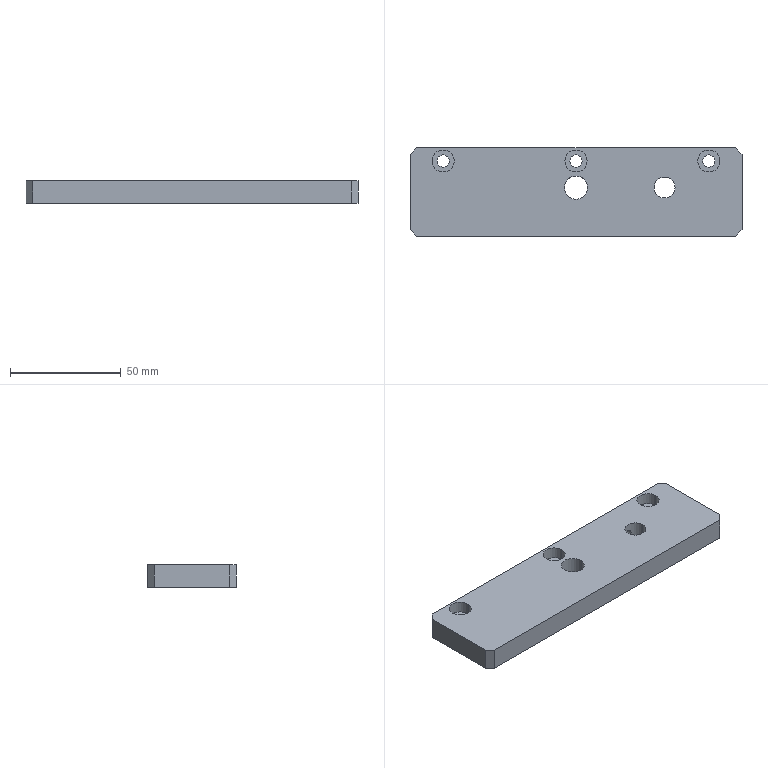Part | SolidWorks | features HoleWzd 3, Chamfer 1, Extrusion 1, ICE 1 | 1 solid | 31 faces | box 150 x 40 x 10 mm | volume 56531 mm3 | cylinder 18 | plane 13 | commonest cylinder face diameters 5.5 x6 10 x6 3.3 x2 9.5 x2 10.5 x2
STEP:
#1=CARTESIAN_POINT('',(40.,6.75,3.35));
#2=VERTEX_POINT('',#1);
#3=CARTESIAN_POINT('',(40.,6.75,6.65));
#4=VERTEX_POINT('',#3);
#5=CARTESIAN_POINT('',(40.,6.75,3.35));
#6=CARTESIAN_POINT('',(39.783,6.75,3.35));
#7=CARTESIAN_POINT('',(39.565,6.734,3.394));
#8=CARTESIAN_POINT('',(39.266,6.694,3.518));
#9=CARTESIAN_POINT('',(39.17,6.678,3.57));
#10=CARTESIAN_POINT('',(38.992,6.643,3.69));
#11=CARTESIAN_POINT('',(38.909,6.624,3.757));
#12=CARTESIAN_POINT('',(38.68,6.566,3.986));
#13=CARTESIAN_POINT('',(38.56,6.527,4.166));
#14=CARTESIAN_POINT('',(38.435,6.485,4.466));
#15=CARTESIAN_POINT('',(38.403,6.474,4.569));
#16=CARTESIAN_POINT('',(38.361,6.458,4.781));
#17=CARTESIAN_POINT('',(38.35,6.454,4.892));
#18=CARTESIAN_POINT('',(38.35,6.454,5.109));
#19=CARTESIAN_POINT('',(38.361,6.458,5.217));
#20=CARTESIAN_POINT('',(38.403,6.474,5.43));
#21=CARTESIAN_POINT('',(38.436,6.485,5.535));
#22=CARTESIAN_POINT('',(38.56,6.527,5.833));
#23=CARTESIAN_POINT('',(38.682,6.566,6.015));
#24=CARTESIAN_POINT('',(38.909,6.624,6.242));
#25=CARTESIAN_POINT('',(38.993,6.643,6.312));
#26=CARTESIAN_POINT('',(39.171,6.678,6.431));
#27=CARTESIAN_POINT('',(39.266,6.694,6.481));
#28=CARTESIAN_POINT('',(39.465,6.721,6.565));
#29=CARTESIAN_POINT('',(39.57,6.732,6.597));
#30=CARTESIAN_POINT('',(39.782,6.746,6.639));
#31=CARTESIAN_POINT('',(39.89,6.75,6.65));
#32=CARTESIAN_POINT('',(40.,6.75,6.65));
#33=B_SPLINE_CURVE_WITH_KNOTS('',3,(#5,#6,#7,#8,#9,#10,#11,#12,#13,#14,#15,#16,#17,#18,#19,#20,#21,#22,#23,#24,#25,#26,#27,#28,#29,#30,#31,#32),.UNSPECIFIED.,.F.,.F.,(4,2,2,2,2,2,2,2,2,2,2,2,2,4),(0.0052,0.005849,0.006174,0.006499,0.007149,0.007474,0.007799,0.008124,0.008448,0.009098,0.009423,0.009748,0.01007,0.0104),.UNSPECIFIED.);
#34=EDGE_CURVE('',#2,#4,#33,.T.);
#35=ORIENTED_EDGE('',*,*,#34,.F.);
#36=CARTESIAN_POINT('',(40.,20.,3.35));
#37=VERTEX_POINT('',#36);
#38=CARTESIAN_POINT('',(40.,20.,3.35));
#39=DIRECTION('',(0.,1.,0.));
#40=VECTOR('',#39,1000.);
#41=LINE('',#38,#40);
#42=EDGE_CURVE('',#2,#37,#41,.T.);
#43=ORIENTED_EDGE('',*,*,#42,.T.);
#44=CARTESIAN_POINT('',(40.,20.,6.65));
#45=VERTEX_POINT('',#44);
#46=CARTESIAN_POINT('',(40.,20.,5.));
#47=DIRECTION('',(0.,1.,0.));
#48=DIRECTION('',(0.,0.,1.));
#49=AXIS2_PLACEMENT_3D('',#46,#47,#48);
#50=CIRCLE('',#49,1.65);
#51=EDGE_CURVE('',#37,#45,#50,.T.);
#52=ORIENTED_EDGE('',*,*,#51,.T.);
#53=CARTESIAN_POINT('',(40.,20.,6.65));
#54=DIRECTION('',(0.,1.,0.));
#55=VECTOR('',#54,1000.);
#56=LINE('',#53,#55);
#57=EDGE_CURVE('',#4,#45,#56,.T.);
#58=ORIENTED_EDGE('',*,*,#57,.F.);
#59=EDGE_LOOP('',(#35,#43,#52,#58));
#60=FACE_OUTER_BOUND('',#59,.T.);
#61=CARTESIAN_POINT('',(40.,20.,5.));
#62=DIRECTION('',(0.,1.,0.));
#63=DIRECTION('',(0.,0.,1.));
#64=AXIS2_PLACEMENT_3D('',#61,#62,#63);
#65=CYLINDRICAL_SURFACE('',#64,1.65);
#66=ADVANCED_FACE('',(#60),#65,.F.);
#67=CARTESIAN_POINT('',(55.,14.,4.6));
#68=VERTEX_POINT('',#67);
#69=CARTESIAN_POINT('',(65.,14.,4.6));
#70=VERTEX_POINT('',#69);
#71=CARTESIAN_POINT('',(60.,14.,4.6));
#72=DIRECTION('',(0.,0.,1.));
#73=DIRECTION('',(1.,0.,0.));
#74=AXIS2_PLACEMENT_3D('',#71,#72,#73);
#75=CIRCLE('',#74,5.);
#76=EDGE_CURVE('',#68,#70,#75,.T.);
#77=ORIENTED_EDGE('',*,*,#76,.F.);
#78=CARTESIAN_POINT('',(55.,14.,10.));
#79=VERTEX_POINT('',#78);
#80=CARTESIAN_POINT('',(55.,14.,10.));
#81=DIRECTION('',(0.,0.,1.));
#82=VECTOR('',#81,1000.);
#83=LINE('',#80,#82);
#84=EDGE_CURVE('',#68,#79,#83,.T.);
#85=ORIENTED_EDGE('',*,*,#84,.T.);
#86=CARTESIAN_POINT('',(65.,14.,10.));
#87=VERTEX_POINT('',#86);
#88=CARTESIAN_POINT('',(60.,14.,10.));
#89=DIRECTION('',(0.,0.,1.));
#90=DIRECTION('',(1.,0.,0.));
#91=AXIS2_PLACEMENT_3D('',#88,#89,#90);
#92=CIRCLE('',#91,5.);
#93=EDGE_CURVE('',#79,#87,#92,.T.);
#94=ORIENTED_EDGE('',*,*,#93,.T.);
#95=CARTESIAN_POINT('',(65.,14.,10.));
#96=DIRECTION('',(0.,0.,1.));
#97=VECTOR('',#96,1000.);
#98=LINE('',#95,#97);
#99=EDGE_CURVE('',#70,#87,#98,.T.);
#100=ORIENTED_EDGE('',*,*,#99,.F.);
#101=EDGE_LOOP('',(#77,#85,#94,#100));
#102=FACE_OUTER_BOUND('',#101,.T.);
#103=CARTESIAN_POINT('',(60.,14.,10.));
#104=DIRECTION('',(0.,0.,1.));
#105=DIRECTION('',(1.,0.,0.));
#106=AXIS2_PLACEMENT_3D('',#103,#104,#105);
#107=CYLINDRICAL_SURFACE('',#106,5.);
#108=ADVANCED_FACE('',(#102),#107,.F.);
#109=CARTESIAN_POINT('',(57.25,14.,0.));
#110=VERTEX_POINT('',#109);
#111=CARTESIAN_POINT('',(62.75,14.,0.));
#112=VERTEX_POINT('',#111);
#113=CARTESIAN_POINT('',(60.,14.,0.));
#114=DIRECTION('',(0.,0.,1.));
#115=DIRECTION('',(1.,0.,0.));
#116=AXIS2_PLACEMENT_3D('',#113,#114,#115);
#117=CIRCLE('',#116,2.75);
#118=EDGE_CURVE('',#110,#112,#117,.T.);
#119=ORIENTED_EDGE('',*,*,#118,.F.);
#120=CARTESIAN_POINT('',(57.25,14.,4.6));
#121=VERTEX_POINT('',#120);
#122=CARTESIAN_POINT('',(57.25,14.,10.));
#123=DIRECTION('',(0.,0.,1.));
#124=VECTOR('',#123,1000.);
#125=LINE('',#122,#124);
#126=EDGE_CURVE('',#110,#121,#125,.T.);
#127=ORIENTED_EDGE('',*,*,#126,.T.);
#128=CARTESIAN_POINT('',(62.75,14.,4.6));
#129=VERTEX_POINT('',#128);
#130=CARTESIAN_POINT('',(60.,14.,4.6));
#131=DIRECTION('',(0.,0.,1.));
#132=DIRECTION('',(1.,0.,0.));
#133=AXIS2_PLACEMENT_3D('',#130,#131,#132);
#134=CIRCLE('',#133,2.75);
#135=EDGE_CURVE('',#121,#129,#134,.T.);
#136=ORIENTED_EDGE('',*,*,#135,.T.);
#137=CARTESIAN_POINT('',(62.75,14.,10.));
#138=DIRECTION('',(0.,0.,1.));
#139=VECTOR('',#138,1000.);
#140=LINE('',#137,#139);
#141=EDGE_CURVE('',#112,#129,#140,.T.);
#142=ORIENTED_EDGE('',*,*,#141,.F.);
#143=EDGE_LOOP('',(#119,#127,#136,#142));
#144=FACE_OUTER_BOUND('',#143,.T.);
#145=CARTESIAN_POINT('',(60.,14.,10.));
#146=DIRECTION('',(0.,0.,1.));
#147=DIRECTION('',(1.,0.,0.));
#148=AXIS2_PLACEMENT_3D('',#145,#146,#147);
#149=CYLINDRICAL_SURFACE('',#148,2.75);
#150=ADVANCED_FACE('',(#144),#149,.F.);
#151=CARTESIAN_POINT('',(-5.,14.,4.6));
#152=VERTEX_POINT('',#151);
#153=CARTESIAN_POINT('',(5.,14.,4.6));
#154=VERTEX_POINT('',#153);
#155=CARTESIAN_POINT('',(0.,14.,4.6));
#156=DIRECTION('',(0.,0.,1.));
#157=DIRECTION('',(1.,0.,0.));
#158=AXIS2_PLACEMENT_3D('',#155,#156,#157);
#159=CIRCLE('',#158,5.);
#160=EDGE_CURVE('',#152,#154,#159,.T.);
#161=ORIENTED_EDGE('',*,*,#160,.F.);
#162=CARTESIAN_POINT('',(-5.,14.,10.));
#163=VERTEX_POINT('',#162);
#164=CARTESIAN_POINT('',(-5.,14.,10.));
#165=DIRECTION('',(0.,0.,1.));
#166=VECTOR('',#165,1000.);
#167=LINE('',#164,#166);
#168=EDGE_CURVE('',#152,#163,#167,.T.);
#169=ORIENTED_EDGE('',*,*,#168,.T.);
#170=CARTESIAN_POINT('',(5.,14.,10.));
#171=VERTEX_POINT('',#170);
#172=CARTESIAN_POINT('',(0.,14.,10.));
#173=DIRECTION('',(0.,0.,1.));
#174=DIRECTION('',(1.,0.,0.));
#175=AXIS2_PLACEMENT_3D('',#172,#173,#174);
#176=CIRCLE('',#175,5.);
#177=EDGE_CURVE('',#163,#171,#176,.T.);
#178=ORIENTED_EDGE('',*,*,#177,.T.);
#179=CARTESIAN_POINT('',(5.,14.,10.));
#180=DIRECTION('',(0.,0.,1.));
#181=VECTOR('',#180,1000.);
#182=LINE('',#179,#181);
#183=EDGE_CURVE('',#154,#171,#182,.T.);
#184=ORIENTED_EDGE('',*,*,#183,.F.);
#185=EDGE_LOOP('',(#161,#169,#178,#184));
#186=FACE_OUTER_BOUND('',#185,.T.);
#187=CARTESIAN_POINT('',(0.,14.,10.));
#188=DIRECTION('',(0.,0.,1.));
#189=DIRECTION('',(1.,0.,0.));
#190=AXIS2_PLACEMENT_3D('',#187,#188,#189);
#191=CYLINDRICAL_SURFACE('',#190,5.);
#192=ADVANCED_FACE('',(#186),#191,.F.);
#193=CARTESIAN_POINT('',(-2.75,14.,0.));
#194=VERTEX_POINT('',#193);
#195=CARTESIAN_POINT('',(2.75,14.,0.));
#196=VERTEX_POINT('',#195);
#197=CARTESIAN_POINT('',(0.,14.,0.));
#198=DIRECTION('',(0.,0.,1.));
#199=DIRECTION('',(1.,0.,0.));
#200=AXIS2_PLACEMENT_3D('',#197,#198,#199);
#201=CIRCLE('',#200,2.75);
#202=EDGE_CURVE('',#194,#196,#201,.T.);
#203=ORIENTED_EDGE('',*,*,#202,.F.);
#204=CARTESIAN_POINT('',(-2.75,14.,4.6));
#205=VERTEX_POINT('',#204);
#206=CARTESIAN_POINT('',(-2.75,14.,10.));
#207=DIRECTION('',(0.,0.,1.));
#208=VECTOR('',#207,1000.);
#209=LINE('',#206,#208);
#210=EDGE_CURVE('',#194,#205,#209,.T.);
#211=ORIENTED_EDGE('',*,*,#210,.T.);
#212=CARTESIAN_POINT('',(2.75,14.,4.6));
#213=VERTEX_POINT('',#212);
#214=CARTESIAN_POINT('',(0.,14.,4.6));
#215=DIRECTION('',(0.,0.,1.));
#216=DIRECTION('',(1.,0.,0.));
#217=AXIS2_PLACEMENT_3D('',#214,#215,#216);
#218=CIRCLE('',#217,2.75);
#219=EDGE_CURVE('',#205,#213,#218,.T.);
#220=ORIENTED_EDGE('',*,*,#219,.T.);
#221=CARTESIAN_POINT('',(2.75,14.,10.));
#222=DIRECTION('',(0.,0.,1.));
#223=VECTOR('',#222,1000.);
#224=LINE('',#221,#223);
#225=EDGE_CURVE('',#196,#213,#224,.T.);
#226=ORIENTED_EDGE('',*,*,#225,.F.);
#227=EDGE_LOOP('',(#203,#211,#220,#226));
#228=FACE_OUTER_BOUND('',#227,.T.);
#229=CARTESIAN_POINT('',(0.,14.,10.));
#230=DIRECTION('',(0.,0.,1.));
#231=DIRECTION('',(1.,0.,0.));
#232=AXIS2_PLACEMENT_3D('',#229,#230,#231);
#233=CYLINDRICAL_SURFACE('',#232,2.75);
#234=ADVANCED_FACE('',(#228),#233,.F.);
#235=CARTESIAN_POINT('',(-65.,14.,4.6));
#236=VERTEX_POINT('',#235);
#237=CARTESIAN_POINT('',(-55.,14.,4.6));
#238=VERTEX_POINT('',#237);
#239=CARTESIAN_POINT('',(-60.,14.,4.6));
#240=DIRECTION('',(0.,0.,1.));
#241=DIRECTION('',(1.,0.,0.));
#242=AXIS2_PLACEMENT_3D('',#239,#240,#241);
#243=CIRCLE('',#242,5.);
#244=EDGE_CURVE('',#236,#238,#243,.T.);
#245=ORIENTED_EDGE('',*,*,#244,.F.);
#246=CARTESIAN_POINT('',(-65.,14.,10.));
#247=VERTEX_POINT('',#246);
#248=CARTESIAN_POINT('',(-65.,14.,10.));
#249=DIRECTION('',(0.,0.,1.));
#250=VECTOR('',#249,1000.);
#251=LINE('',#248,#250);
#252=EDGE_CURVE('',#236,#247,#251,.T.);
#253=ORIENTED_EDGE('',*,*,#252,.T.);
#254=CARTESIAN_POINT('',(-55.,14.,10.));
#255=VERTEX_POINT('',#254);
#256=CARTESIAN_POINT('',(-60.,14.,10.));
#257=DIRECTION('',(0.,0.,1.));
#258=DIRECTION('',(1.,0.,0.));
#259=AXIS2_PLACEMENT_3D('',#256,#257,#258);
#260=CIRCLE('',#259,5.);
#261=EDGE_CURVE('',#247,#255,#260,.T.);
#262=ORIENTED_EDGE('',*,*,#261,.T.);
#263=CARTESIAN_POINT('',(-55.,14.,10.));
#264=DIRECTION('',(0.,0.,1.));
#265=VECTOR('',#264,1000.);
#266=LINE('',#263,#265);
#267=EDGE_CURVE('',#238,#255,#266,.T.);
#268=ORIENTED_EDGE('',*,*,#267,.F.);
#269=EDGE_LOOP('',(#245,#253,#262,#268));
#270=FACE_OUTER_BOUND('',#269,.T.);
#271=CARTESIAN_POINT('',(-60.,14.,10.));
#272=DIRECTION('',(0.,0.,1.));
#273=DIRECTION('',(1.,0.,0.));
#274=AXIS2_PLACEMENT_3D('',#271,#272,#273);
#275=CYLINDRICAL_SURFACE('',#274,5.);
#276=ADVANCED_FACE('',(#270),#275,.F.);
#277=CARTESIAN_POINT('',(-62.75,14.,0.));
#278=VERTEX_POINT('',#277);
#279=CARTESIAN_POINT('',(-57.25,14.,0.));
#280=VERTEX_POINT('',#279);
#281=CARTESIAN_POINT('',(-60.,14.,0.));
#282=DIRECTION('',(0.,0.,1.));
#283=DIRECTION('',(1.,0.,0.));
#284=AXIS2_PLACEMENT_3D('',#281,#282,#283);
#285=CIRCLE('',#284,2.75);
#286=EDGE_CURVE('',#278,#280,#285,.T.);
#287=ORIENTED_EDGE('',*,*,#286,.F.);
#288=CARTESIAN_POINT('',(-62.75,14.,4.6));
#289=VERTEX_POINT('',#288);
#290=CARTESIAN_POINT('',(-62.75,14.,10.));
#291=DIRECTION('',(0.,0.,1.));
#292=VECTOR('',#291,1000.);
#293=LINE('',#290,#292);
#294=EDGE_CURVE('',#278,#289,#293,.T.);
#295=ORIENTED_EDGE('',*,*,#294,.T.);
#296=CARTESIAN_POINT('',(-57.25,14.,4.6));
#297=VERTEX_POINT('',#296);
#298=CARTESIAN_POINT('',(-60.,14.,4.6));
#299=DIRECTION('',(0.,0.,1.));
#300=DIRECTION('',(1.,0.,0.));
#301=AXIS2_PLACEMENT_3D('',#298,#299,#300);
#302=CIRCLE('',#301,2.75);
#303=EDGE_CURVE('',#289,#297,#302,.T.);
#304=ORIENTED_EDGE('',*,*,#303,.T.);
#305=CARTESIAN_POINT('',(-57.25,14.,10.));
#306=DIRECTION('',(0.,0.,1.));
#307=VECTOR('',#306,1000.);
#308=LINE('',#305,#307);
#309=EDGE_CURVE('',#280,#297,#308,.T.);
#310=ORIENTED_EDGE('',*,*,#309,.F.);
#311=EDGE_LOOP('',(#287,#295,#304,#310));
#312=FACE_OUTER_BOUND('',#311,.T.);
#313=CARTESIAN_POINT('',(-60.,14.,10.));
#314=DIRECTION('',(0.,0.,1.));
#315=DIRECTION('',(1.,0.,0.));
#316=AXIS2_PLACEMENT_3D('',#313,#314,#315);
#317=CYLINDRICAL_SURFACE('',#316,2.75);
#318=ADVANCED_FACE('',(#312),#317,.F.);
#319=CARTESIAN_POINT('',(-5.25,2.,0.));
#320=VERTEX_POINT('',#319);
#321=CARTESIAN_POINT('',(5.25,2.,0.));
#322=VERTEX_POINT('',#321);
#323=CARTESIAN_POINT('',(0.,2.,0.));
#324=DIRECTION('',(0.,0.,1.));
#325=DIRECTION('',(1.,0.,0.));
#326=AXIS2_PLACEMENT_3D('',#323,#324,#325);
#327=CIRCLE('',#326,5.25);
#328=EDGE_CURVE('',#320,#322,#327,.T.);
#329=ORIENTED_EDGE('',*,*,#328,.F.);
#330=CARTESIAN_POINT('',(-5.25,2.,10.));
#331=VERTEX_POINT('',#330);
#332=CARTESIAN_POINT('',(-5.25,2.,10.));
#333=DIRECTION('',(0.,0.,1.));
#334=VECTOR('',#333,1000.);
#335=LINE('',#332,#334);
#336=EDGE_CURVE('',#320,#331,#335,.T.);
#337=ORIENTED_EDGE('',*,*,#336,.T.);
#338=CARTESIAN_POINT('',(5.25,2.,10.));
#339=VERTEX_POINT('',#338);
#340=CARTESIAN_POINT('',(0.,2.,10.));
#341=DIRECTION('',(0.,0.,1.));
#342=DIRECTION('',(1.,0.,0.));
#343=AXIS2_PLACEMENT_3D('',#340,#341,#342);
#344=CIRCLE('',#343,5.25);
#345=EDGE_CURVE('',#331,#339,#344,.T.);
#346=ORIENTED_EDGE('',*,*,#345,.T.);
#347=CARTESIAN_POINT('',(5.25,2.,10.));
#348=DIRECTION('',(0.,0.,1.));
#349=VECTOR('',#348,1000.);
#350=LINE('',#347,#349);
#351=EDGE_CURVE('',#322,#339,#350,.T.);
#352=ORIENTED_EDGE('',*,*,#351,.F.);
#353=EDGE_LOOP('',(#329,#337,#346,#352));
#354=FACE_OUTER_BOUND('',#353,.T.);
#355=CARTESIAN_POINT('',(0.,2.,10.));
#356=DIRECTION('',(0.,0.,1.));
#357=DIRECTION('',(1.,0.,0.));
#358=AXIS2_PLACEMENT_3D('',#355,#356,#357);
#359=CYLINDRICAL_SURFACE('',#358,5.25);
#360=ADVANCED_FACE('',(#354),#359,.F.);
#361=CARTESIAN_POINT('',(35.25,2.,0.));
#362=VERTEX_POINT('',#361);
#363=CARTESIAN_POINT('',(44.75,2.,0.));
#364=VERTEX_POINT('',#363);
#365=CARTESIAN_POINT('',(40.,2.,0.));
#366=DIRECTION('',(0.,0.,1.));
#367=DIRECTION('',(1.,0.,0.));
#368=AXIS2_PLACEMENT_3D('',#365,#366,#367);
#369=CIRCLE('',#368,4.75);
#370=EDGE_CURVE('',#362,#364,#369,.T.);
#371=ORIENTED_EDGE('',*,*,#370,.F.);
#372=CARTESIAN_POINT('',(35.25,2.,10.));
#373=VERTEX_POINT('',#372);
#374=CARTESIAN_POINT('',(35.25,2.,0.));
#375=DIRECTION('',(0.,0.,1.));
#376=VECTOR('',#375,1000.);
#377=LINE('',#374,#376);
#378=EDGE_CURVE('',#362,#373,#377,.T.);
#379=ORIENTED_EDGE('',*,*,#378,.T.);
#380=CARTESIAN_POINT('',(44.75,2.,10.));
#381=VERTEX_POINT('',#380);
#382=CARTESIAN_POINT('',(40.,2.,10.));
#383=DIRECTION('',(0.,0.,1.));
#384=DIRECTION('',(1.,0.,0.));
#385=AXIS2_PLACEMENT_3D('',#382,#383,#384);
#386=CIRCLE('',#385,4.75);
#387=EDGE_CURVE('',#373,#381,#386,.T.);
#388=ORIENTED_EDGE('',*,*,#387,.T.);
#389=CARTESIAN_POINT('',(44.75,2.,0.));
#390=DIRECTION('',(0.,0.,1.));
#391=VECTOR('',#390,1000.);
#392=LINE('',#389,#391);
#393=EDGE_CURVE('',#364,#381,#392,.T.);
#394=ORIENTED_EDGE('',*,*,#393,.F.);
#395=EDGE_LOOP('',(#371,#379,#388,#394));
#396=FACE_OUTER_BOUND('',#395,.T.);
#397=CARTESIAN_POINT('',(40.,2.,0.));
#398=DIRECTION('',(0.,0.,1.));
#399=DIRECTION('',(1.,0.,0.));
#400=AXIS2_PLACEMENT_3D('',#397,#398,#399);
#401=CYLINDRICAL_SURFACE('',#400,4.75);
#402=ADVANCED_FACE('',(#396),#401,.F.);
#403=CARTESIAN_POINT('',(75.,-17.,10.));
#404=VERTEX_POINT('',#403);
#405=CARTESIAN_POINT('',(75.,17.,10.));
#406=VERTEX_POINT('',#405);
#407=CARTESIAN_POINT('',(75.,20.,10.));
#408=DIRECTION('',(0.,1.,0.));
#409=VECTOR('',#408,1000.);
#410=LINE('',#407,#409);
#411=EDGE_CURVE('',#404,#406,#410,.T.);
#412=ORIENTED_EDGE('',*,*,#411,.F.);
#413=CARTESIAN_POINT('',(75.,-17.,0.));
#414=VERTEX_POINT('',#413);
#415=CARTESIAN_POINT('',(75.,-17.,10.));
#416=DIRECTION('',(0.,0.,-1.));
#417=VECTOR('',#416,1000.);
#418=LINE('',#415,#417);
#419=EDGE_CURVE('',#404,#414,#418,.T.);
#420=ORIENTED_EDGE('',*,*,#419,.T.);
#421=CARTESIAN_POINT('',(75.,17.,0.));
#422=VERTEX_POINT('',#421);
#423=CARTESIAN_POINT('',(75.,20.,0.));
#424=DIRECTION('',(0.,1.,0.));
#425=VECTOR('',#424,1000.);
#426=LINE('',#423,#425);
#427=EDGE_CURVE('',#414,#422,#426,.T.);
#428=ORIENTED_EDGE('',*,*,#427,.T.);
#429=CARTESIAN_POINT('',(75.,17.,10.));
#430=DIRECTION('',(0.,0.,1.));
#431=VECTOR('',#430,1000.);
#432=LINE('',#429,#431);
#433=EDGE_CURVE('',#422,#406,#432,.T.);
#434=ORIENTED_EDGE('',*,*,#433,.T.);
#435=EDGE_LOOP('',(#412,#420,#428,#434));
#436=FACE_OUTER_BOUND('',#435,.T.);
#437=CARTESIAN_POINT('',(75.,20.,10.));
#438=DIRECTION('',(-1.,0.,0.));
#439=DIRECTION('',(0.,0.,1.));
#440=AXIS2_PLACEMENT_3D('',#437,#438,#439);
#441=PLANE('',#440);
#442=ADVANCED_FACE('',(#436),#441,.F.);
#443=CARTESIAN_POINT('',(40.,20.,5.));
#444=DIRECTION('',(0.,1.,0.));
#445=DIRECTION('',(0.,0.,1.));
#446=AXIS2_PLACEMENT_3D('',#443,#444,#445);
#447=CIRCLE('',#446,1.65);
#448=EDGE_CURVE('',#45,#37,#447,.T.);
#449=ORIENTED_EDGE('',*,*,#448,.F.);
#450=ORIENTED_EDGE('',*,*,#51,.F.);
#451=EDGE_LOOP('',(#449,#450));
#452=FACE_BOUND('',#451,.T.);
#453=CARTESIAN_POINT('',(72.,20.,0.));
#454=VERTEX_POINT('',#453);
#455=CARTESIAN_POINT('',(-72.,20.,0.));
#456=VERTEX_POINT('',#455);
#457=CARTESIAN_POINT('',(-75.,20.,0.));
#458=DIRECTION('',(-1.,0.,0.));
#459=VECTOR('',#458,1000.);
#460=LINE('',#457,#459);
#461=EDGE_CURVE('',#454,#456,#460,.T.);
#462=ORIENTED_EDGE('',*,*,#461,.T.);
#463=CARTESIAN_POINT('',(-72.,20.,10.));
#464=VERTEX_POINT('',#463);
#465=CARTESIAN_POINT('',(-72.,20.,10.));
#466=DIRECTION('',(0.,0.,1.));
#467=VECTOR('',#466,1000.);
#468=LINE('',#465,#467);
#469=EDGE_CURVE('',#456,#464,#468,.T.);
#470=ORIENTED_EDGE('',*,*,#469,.T.);
#471=CARTESIAN_POINT('',(72.,20.,10.));
#472=VERTEX_POINT('',#471);
#473=CARTESIAN_POINT('',(-75.,20.,10.));
#474=DIRECTION('',(-1.,0.,0.));
#475=VECTOR('',#474,1000.);
#476=LINE('',#473,#475);
#477=EDGE_CURVE('',#472,#464,#476,.T.);
#478=ORIENTED_EDGE('',*,*,#477,.F.);
#479=CARTESIAN_POINT('',(72.,20.,10.));
#480=DIRECTION('',(0.,0.,-1.));
#481=VECTOR('',#480,1000.);
#482=LINE('',#479,#481);
#483=EDGE_CURVE('',#472,#454,#482,.T.);
#484=ORIENTED_EDGE('',*,*,#483,.T.);
#485=EDGE_LOOP('',(#462,#470,#478,#484));
#486=FACE_OUTER_BOUND('',#485,.T.);
#487=CARTESIAN_POINT('',(-75.,20.,10.));
#488=DIRECTION('',(0.,-1.,0.));
#489=DIRECTION('',(0.,0.,-1.));
#490=AXIS2_PLACEMENT_3D('',#487,#488,#489);
#491=PLANE('',#490);
#492=ADVANCED_FACE('',(#452,#486),#491,.F.);
#493=CARTESIAN_POINT('',(-75.,17.,0.));
#494=VERTEX_POINT('',#493);
#495=CARTESIAN_POINT('',(-75.,-17.,0.));
#496=VERTEX_POINT('',#495);
#497=CARTESIAN_POINT('',(-75.,20.,0.));
#498=DIRECTION('',(0.,-1.,0.));
#499=VECTOR('',#498,1000.);
#500=LINE('',#497,#499);
#501=EDGE_CURVE('',#494,#496,#500,.T.);
#502=ORIENTED_EDGE('',*,*,#501,.T.);
#503=CARTESIAN_POINT('',(-75.,-17.,10.));
#504=VERTEX_POINT('',#503);
#505=CARTESIAN_POINT('',(-75.,-17.,10.));
#506=DIRECTION('',(0.,0.,1.));
#507=VECTOR('',#506,1000.);
#508=LINE('',#505,#507);
#509=EDGE_CURVE('',#496,#504,#508,.T.);
#510=ORIENTED_EDGE('',*,*,#509,.T.);
#511=CARTESIAN_POINT('',(-75.,17.,10.));
#512=VERTEX_POINT('',#511);
#513=CARTESIAN_POINT('',(-75.,20.,10.));
#514=DIRECTION('',(0.,-1.,0.));
#515=VECTOR('',#514,1000.);
#516=LINE('',#513,#515);
#517=EDGE_CURVE('',#512,#504,#516,.T.);
#518=ORIENTED_EDGE('',*,*,#517,.F.);
#519=CARTESIAN_POINT('',(-75.,17.,10.));
#520=DIRECTION('',(0.,0.,-1.));
#521=VECTOR('',#520,1000.);
#522=LINE('',#519,#521);
#523=EDGE_CURVE('',#512,#494,#522,.T.);
#524=ORIENTED_EDGE('',*,*,#523,.T.);
#525=EDGE_LOOP('',(#502,#510,#518,#524));
#526=FACE_OUTER_BOUND('',#525,.T.);
#527=CARTESIAN_POINT('',(-75.,20.,10.));
#528=DIRECTION('',(1.,0.,0.));
#529=DIRECTION('',(0.,0.,-1.));
#530=AXIS2_PLACEMENT_3D('',#527,#528,#529);
#531=PLANE('',#530);
#532=ADVANCED_FACE('',(#526),#531,.F.);
#533=CARTESIAN_POINT('',(-72.,-20.,0.));
#534=VERTEX_POINT('',#533);
#535=CARTESIAN_POINT('',(72.,-20.,0.));
#536=VERTEX_POINT('',#535);
#537=CARTESIAN_POINT('',(-75.,-20.,0.));
#538=DIRECTION('',(1.,0.,0.));
#539=VECTOR('',#538,1000.);
#540=LINE('',#537,#539);
#541=EDGE_CURVE('',#534,#536,#540,.T.);
#542=ORIENTED_EDGE('',*,*,#541,.T.);
#543=CARTESIAN_POINT('',(72.,-20.,10.));
#544=VERTEX_POINT('',#543);
#545=CARTESIAN_POINT('',(72.,-20.,10.));
#546=DIRECTION('',(0.,0.,1.));
#547=VECTOR('',#546,1000.);
#548=LINE('',#545,#547);
#549=EDGE_CURVE('',#536,#544,#548,.T.);
#550=ORIENTED_EDGE('',*,*,#549,.T.);
#551=CARTESIAN_POINT('',(-72.,-20.,10.));
#552=VERTEX_POINT('',#551);
#553=CARTESIAN_POINT('',(-75.,-20.,10.));
#554=DIRECTION('',(1.,0.,0.));
#555=VECTOR('',#554,1000.);
#556=LINE('',#553,#555);
#557=EDGE_CURVE('',#552,#544,#556,.T.);
#558=ORIENTED_EDGE('',*,*,#557,.F.);
#559=CARTESIAN_POINT('',(-72.,-20.,10.));
#560=DIRECTION('',(0.,0.,-1.));
#561=VECTOR('',#560,1000.);
#562=LINE('',#559,#561);
#563=EDGE_CURVE('',#552,#534,#562,.T.);
#564=ORIENTED_EDGE('',*,*,#563,.T.);
#565=EDGE_LOOP('',(#542,#550,#558,#564));
#566=FACE_OUTER_BOUND('',#565,.T.);
#567=CARTESIAN_POINT('',(-75.,-20.,10.));
#568=DIRECTION('',(0.,1.,0.));
#569=DIRECTION('',(0.,0.,1.));
#570=AXIS2_PLACEMENT_3D('',#567,#568,#569);
#571=PLANE('',#570);
#572=ADVANCED_FACE('',(#566),#571,.F.);
#573=CARTESIAN_POINT('',(60.,14.,10.));
#574=DIRECTION('',(0.,0.,1.));
#575=DIRECTION('',(1.,0.,0.));
#576=AXIS2_PLACEMENT_3D('',#573,#574,#575);
#577=CIRCLE('',#576,5.);
#578=EDGE_CURVE('',#87,#79,#577,.T.);
#579=ORIENTED_EDGE('',*,*,#578,.F.);
#580=ORIENTED_EDGE('',*,*,#93,.F.);
#581=EDGE_LOOP('',(#579,#580));
#582=FACE_BOUND('',#581,.T.);
#583=CARTESIAN_POINT('',(0.,14.,10.));
#584=DIRECTION('',(0.,0.,1.));
#585=DIRECTION('',(1.,0.,0.));
#586=AXIS2_PLACEMENT_3D('',#583,#584,#585);
#587=CIRCLE('',#586,5.);
#588=EDGE_CURVE('',#171,#163,#587,.T.);
#589=ORIENTED_EDGE('',*,*,#588,.F.);
#590=ORIENTED_EDGE('',*,*,#177,.F.);
#591=EDGE_LOOP('',(#589,#590));
#592=FACE_BOUND('',#591,.T.);
#593=CARTESIAN_POINT('',(-60.,14.,10.));
#594=DIRECTION('',(0.,0.,1.));
#595=DIRECTION('',(1.,0.,0.));
#596=AXIS2_PLACEMENT_3D('',#593,#594,#595);
#597=CIRCLE('',#596,5.);
#598=EDGE_CURVE('',#255,#247,#597,.T.);
#599=ORIENTED_EDGE('',*,*,#598,.F.);
#600=ORIENTED_EDGE('',*,*,#261,.F.);
#601=EDGE_LOOP('',(#599,#600));
#602=FACE_BOUND('',#601,.T.);
#603=CARTESIAN_POINT('',(0.,2.,10.));
#604=DIRECTION('',(0.,0.,1.));
#605=DIRECTION('',(1.,0.,0.));
#606=AXIS2_PLACEMENT_3D('',#603,#604,#605);
#607=CIRCLE('',#606,5.25);
#608=EDGE_CURVE('',#339,#331,#607,.T.);
#609=ORIENTED_EDGE('',*,*,#608,.F.);
#610=ORIENTED_EDGE('',*,*,#345,.F.);
#611=EDGE_LOOP('',(#609,#610));
#612=FACE_BOUND('',#611,.T.);
#613=CARTESIAN_POINT('',(40.,2.,10.));
#614=DIRECTION('',(0.,0.,1.));
#615=DIRECTION('',(1.,0.,0.));
#616=AXIS2_PLACEMENT_3D('',#613,#614,#615);
#617=CIRCLE('',#616,4.75);
#618=EDGE_CURVE('',#381,#373,#617,.T.);
#619=ORIENTED_EDGE('',*,*,#618,.F.);
#620=ORIENTED_EDGE('',*,*,#387,.F.);
#621=EDGE_LOOP('',(#619,#620));
#622=FACE_BOUND('',#621,.T.);
#623=ORIENTED_EDGE('',*,*,#557,.T.);
#624=CARTESIAN_POINT('',(46.,-46.,10.));
#625=DIRECTION('',(0.7071,0.7071,0.));
#626=VECTOR('',#625,1000.);
#627=LINE('',#624,#626);
#628=EDGE_CURVE('',#544,#404,#627,.T.);
#629=ORIENTED_EDGE('',*,*,#628,.T.);
#630=ORIENTED_EDGE('',*,*,#411,.T.);
#631=CARTESIAN_POINT('',(46.,46.,10.));
#632=DIRECTION('',(-0.7071,0.7071,0.));
#633=VECTOR('',#632,1000.);
#634=LINE('',#631,#633);
#635=EDGE_CURVE('',#406,#472,#634,.T.);
#636=ORIENTED_EDGE('',*,*,#635,.T.);
#637=ORIENTED_EDGE('',*,*,#477,.T.);
#638=CARTESIAN_POINT('',(-46.,46.,10.));
#639=DIRECTION('',(-0.7071,-0.7071,0.));
#640=VECTOR('',#639,1000.);
#641=LINE('',#638,#640);
#642=EDGE_CURVE('',#464,#512,#641,.T.);
#643=ORIENTED_EDGE('',*,*,#642,.T.);
#644=ORIENTED_EDGE('',*,*,#517,.T.);
#645=CARTESIAN_POINT('',(-46.,-46.,10.));
#646=DIRECTION('',(0.7071,-0.7071,0.));
#647=VECTOR('',#646,1000.);
#648=LINE('',#645,#647);
#649=EDGE_CURVE('',#504,#552,#648,.T.);
#650=ORIENTED_EDGE('',*,*,#649,.T.);
#651=EDGE_LOOP('',(#623,#629,#630,#636,#637,#643,#644,#650));
#652=FACE_OUTER_BOUND('',#651,.T.);
#653=CARTESIAN_POINT('',(0.,0.,10.));
#654=DIRECTION('',(0.,0.,1.));
#655=DIRECTION('',(1.,0.,0.));
#656=AXIS2_PLACEMENT_3D('',#653,#654,#655);
#657=PLANE('',#656);
#658=ADVANCED_FACE('',(#582,#592,#602,#612,#622,#652),#657,.T.);
#659=CARTESIAN_POINT('',(60.,14.,0.));
#660=DIRECTION('',(0.,0.,1.));
#661=DIRECTION('',(1.,0.,0.));
#662=AXIS2_PLACEMENT_3D('',#659,#660,#661);
#663=CIRCLE('',#662,2.75);
#664=EDGE_CURVE('',#112,#110,#663,.T.);
#665=ORIENTED_EDGE('',*,*,#664,.T.);
#666=ORIENTED_EDGE('',*,*,#118,.T.);
#667=EDGE_LOOP('',(#665,#666));
#668=FACE_BOUND('',#667,.T.);
#669=CARTESIAN_POINT('',(0.,14.,0.));
#670=DIRECTION('',(0.,0.,1.));
#671=DIRECTION('',(1.,0.,0.));
#672=AXIS2_PLACEMENT_3D('',#669,#670,#671);
#673=CIRCLE('',#672,2.75);
#674=EDGE_CURVE('',#196,#194,#673,.T.);
#675=ORIENTED_EDGE('',*,*,#674,.T.);
#676=ORIENTED_EDGE('',*,*,#202,.T.);
#677=EDGE_LOOP('',(#675,#676));
#678=FACE_BOUND('',#677,.T.);
#679=CARTESIAN_POINT('',(-60.,14.,0.));
#680=DIRECTION('',(0.,0.,1.));
#681=DIRECTION('',(1.,0.,0.));
#682=AXIS2_PLACEMENT_3D('',#679,#680,#681);
#683=CIRCLE('',#682,2.75);
#684=EDGE_CURVE('',#280,#278,#683,.T.);
#685=ORIENTED_EDGE('',*,*,#684,.T.);
#686=ORIENTED_EDGE('',*,*,#286,.T.);
#687=EDGE_LOOP('',(#685,#686));
#688=FACE_BOUND('',#687,.T.);
#689=CARTESIAN_POINT('',(0.,2.,0.));
#690=DIRECTION('',(0.,0.,1.));
#691=DIRECTION('',(1.,0.,0.));
#692=AXIS2_PLACEMENT_3D('',#689,#690,#691);
#693=CIRCLE('',#692,5.25);
#694=EDGE_CURVE('',#322,#320,#693,.T.);
#695=ORIENTED_EDGE('',*,*,#694,.T.);
#696=ORIENTED_EDGE('',*,*,#328,.T.);
#697=EDGE_LOOP('',(#695,#696));
#698=FACE_BOUND('',#697,.T.);
#699=CARTESIAN_POINT('',(40.,2.,0.));
#700=DIRECTION('',(0.,0.,1.));
#701=DIRECTION('',(1.,0.,0.));
#702=AXIS2_PLACEMENT_3D('',#699,#700,#701);
#703=CIRCLE('',#702,4.75);
#704=EDGE_CURVE('',#364,#362,#703,.T.);
#705=ORIENTED_EDGE('',*,*,#704,.T.);
#706=ORIENTED_EDGE('',*,*,#370,.T.);
#707=EDGE_LOOP('',(#705,#706));
#708=FACE_BOUND('',#707,.T.);
#709=ORIENTED_EDGE('',*,*,#427,.F.);
#710=CARTESIAN_POINT('',(75.,-17.,0.));
#711=DIRECTION('',(-0.7071,-0.7071,0.));
#712=VECTOR('',#711,1000.);
#713=LINE('',#710,#712);
#714=EDGE_CURVE('',#414,#536,#713,.T.);
#715=ORIENTED_EDGE('',*,*,#714,.T.);
#716=ORIENTED_EDGE('',*,*,#541,.F.);
#717=CARTESIAN_POINT('',(-72.,-20.,0.));
#718=DIRECTION('',(-0.7071,0.7071,0.));
#719=VECTOR('',#718,1000.);
#720=LINE('',#717,#719);
#721=EDGE_CURVE('',#534,#496,#720,.T.);
#722=ORIENTED_EDGE('',*,*,#721,.T.);
#723=ORIENTED_EDGE('',*,*,#501,.F.);
#724=CARTESIAN_POINT('',(-75.,17.,0.));
#725=DIRECTION('',(0.7071,0.7071,0.));
#726=VECTOR('',#725,1000.);
#727=LINE('',#724,#726);
#728=EDGE_CURVE('',#494,#456,#727,.T.);
#729=ORIENTED_EDGE('',*,*,#728,.T.);
#730=ORIENTED_EDGE('',*,*,#461,.F.);
#731=CARTESIAN_POINT('',(72.,20.,0.));
#732=DIRECTION('',(0.7071,-0.7071,0.));
#733=VECTOR('',#732,1000.);
#734=LINE('',#731,#733);
#735=EDGE_CURVE('',#454,#422,#734,.T.);
#736=ORIENTED_EDGE('',*,*,#735,.T.);
#737=EDGE_LOOP('',(#709,#715,#716,#722,#723,#729,#730,#736));
#738=FACE_OUTER_BOUND('',#737,.T.);
#739=CARTESIAN_POINT('',(0.,0.,0.));
#740=DIRECTION('',(0.,0.,1.));
#741=DIRECTION('',(1.,0.,0.));
#742=AXIS2_PLACEMENT_3D('',#739,#740,#741);
#743=PLANE('',#742);
#744=ADVANCED_FACE('',(#668,#678,#688,#698,#708,#738),#743,.F.);
#745=ORIENTED_EDGE('',*,*,#378,.F.);
#746=ORIENTED_EDGE('',*,*,#704,.F.);
#747=ORIENTED_EDGE('',*,*,#393,.T.);
#748=ORIENTED_EDGE('',*,*,#618,.T.);
#749=EDGE_LOOP('',(#745,#746,#747,#748));
#750=FACE_OUTER_BOUND('',#749,.T.);
#751=CARTESIAN_POINT('',(40.,6.75,6.65));
#752=CARTESIAN_POINT('',(40.11,6.75,6.65));
#753=CARTESIAN_POINT('',(40.218,6.746,6.639));
#754=CARTESIAN_POINT('',(40.43,6.732,6.597));
#755=CARTESIAN_POINT('',(40.535,6.721,6.565));
#756=CARTESIAN_POINT('',(40.735,6.694,6.481));
#757=CARTESIAN_POINT('',(40.829,6.678,6.431));
#758=CARTESIAN_POINT('',(41.008,6.643,6.311));
#759=CARTESIAN_POINT('',(41.092,6.623,6.242));
#760=CARTESIAN_POINT('',(41.318,6.566,6.015));
#761=CARTESIAN_POINT('',(41.441,6.527,5.833));
#762=CARTESIAN_POINT('',(41.564,6.485,5.535));
#763=CARTESIAN_POINT('',(41.597,6.474,5.43));
#764=CARTESIAN_POINT('',(41.639,6.458,5.217));
#765=CARTESIAN_POINT('',(41.65,6.454,5.109));
#766=CARTESIAN_POINT('',(41.65,6.454,4.892));
#767=CARTESIAN_POINT('',(41.639,6.458,4.782));
#768=CARTESIAN_POINT('',(41.597,6.474,4.57));
#769=CARTESIAN_POINT('',(41.565,6.485,4.466));
#770=CARTESIAN_POINT('',(41.44,6.527,4.165));
#771=CARTESIAN_POINT('',(41.318,6.566,3.984));
#772=CARTESIAN_POINT('',(41.09,6.624,3.757));
#773=CARTESIAN_POINT('',(41.008,6.643,3.689));
#774=CARTESIAN_POINT('',(40.83,6.678,3.57));
#775=CARTESIAN_POINT('',(40.733,6.694,3.518));
#776=CARTESIAN_POINT('',(40.435,6.734,3.394));
#777=CARTESIAN_POINT('',(40.217,6.75,3.35));
#778=CARTESIAN_POINT('',(40.,6.75,3.35));
#779=B_SPLINE_CURVE_WITH_KNOTS('',3,(#751,#752,#753,#754,#755,#756,#757,#758,#759,#760,#761,#762,#763,#764,#765,#766,#767,#768,#769,#770,#771,#772,#773,#774,#775,#776,#777,#778),.UNSPECIFIED.,.F.,.F.,(4,2,2,2,2,2,2,2,2,2,2,2,2,4),(0.,0.000325,0.0006499,0.0009749,0.0013,0.00195,0.002275,0.0026,0.002925,0.00325,0.0039,0.004225,0.00455,0.0052),.UNSPECIFIED.);
#780=EDGE_CURVE('',#4,#2,#779,.T.);
#781=ORIENTED_EDGE('',*,*,#780,.T.);
#782=ORIENTED_EDGE('',*,*,#34,.T.);
#783=EDGE_LOOP('',(#781,#782));
#784=FACE_BOUND('',#783,.T.);
#785=CARTESIAN_POINT('',(40.,2.,0.));
#786=DIRECTION('',(0.,0.,1.));
#787=DIRECTION('',(1.,0.,0.));
#788=AXIS2_PLACEMENT_3D('',#785,#786,#787);
#789=CYLINDRICAL_SURFACE('',#788,4.75);
#790=ADVANCED_FACE('',(#750,#784),#789,.F.);
#791=ORIENTED_EDGE('',*,*,#336,.F.);
#792=ORIENTED_EDGE('',*,*,#694,.F.);
#793=ORIENTED_EDGE('',*,*,#351,.T.);
#794=ORIENTED_EDGE('',*,*,#608,.T.);
#795=EDGE_LOOP('',(#791,#792,#793,#794));
#796=FACE_OUTER_BOUND('',#795,.T.);
#797=CARTESIAN_POINT('',(0.,2.,10.));
#798=DIRECTION('',(0.,0.,1.));
#799=DIRECTION('',(1.,0.,0.));
#800=AXIS2_PLACEMENT_3D('',#797,#798,#799);
#801=CYLINDRICAL_SURFACE('',#800,5.25);
#802=ADVANCED_FACE('',(#796),#801,.F.);
#803=ORIENTED_EDGE('',*,*,#294,.F.);
#804=ORIENTED_EDGE('',*,*,#684,.F.);
#805=ORIENTED_EDGE('',*,*,#309,.T.);
#806=CARTESIAN_POINT('',(-60.,14.,4.6));
#807=DIRECTION('',(0.,0.,1.));
#808=DIRECTION('',(1.,0.,0.));
#809=AXIS2_PLACEMENT_3D('',#806,#807,#808);
#810=CIRCLE('',#809,2.75);
#811=EDGE_CURVE('',#297,#289,#810,.T.);
#812=ORIENTED_EDGE('',*,*,#811,.T.);
#813=EDGE_LOOP('',(#803,#804,#805,#812));
#814=FACE_OUTER_BOUND('',#813,.T.);
#815=CARTESIAN_POINT('',(-60.,14.,10.));
#816=DIRECTION('',(0.,0.,1.));
#817=DIRECTION('',(1.,0.,0.));
#818=AXIS2_PLACEMENT_3D('',#815,#816,#817);
#819=CYLINDRICAL_SURFACE('',#818,2.75);
#820=ADVANCED_FACE('',(#814),#819,.F.);
#821=ORIENTED_EDGE('',*,*,#811,.F.);
#822=ORIENTED_EDGE('',*,*,#303,.F.);
#823=EDGE_LOOP('',(#821,#822));
#824=FACE_BOUND('',#823,.T.);
#825=CARTESIAN_POINT('',(-60.,14.,4.6));
#826=DIRECTION('',(0.,0.,1.));
#827=DIRECTION('',(1.,0.,0.));
#828=AXIS2_PLACEMENT_3D('',#825,#826,#827);
#829=CIRCLE('',#828,5.);
#830=EDGE_CURVE('',#238,#236,#829,.T.);
#831=ORIENTED_EDGE('',*,*,#830,.T.);
#832=ORIENTED_EDGE('',*,*,#244,.T.);
#833=EDGE_LOOP('',(#831,#832));
#834=FACE_OUTER_BOUND('',#833,.T.);
#835=CARTESIAN_POINT('',(-57.25,14.,4.6));
#836=DIRECTION('',(0.,0.,-1.));
#837=DIRECTION('',(-1.,0.,0.));
#838=AXIS2_PLACEMENT_3D('',#835,#836,#837);
#839=PLANE('',#838);
#840=ADVANCED_FACE('',(#824,#834),#839,.F.);
#841=ORIENTED_EDGE('',*,*,#252,.F.);
#842=ORIENTED_EDGE('',*,*,#830,.F.);
#843=ORIENTED_EDGE('',*,*,#267,.T.);
#844=ORIENTED_EDGE('',*,*,#598,.T.);
#845=EDGE_LOOP('',(#841,#842,#843,#844));
#846=FACE_OUTER_BOUND('',#845,.T.);
#847=CARTESIAN_POINT('',(-60.,14.,10.));
#848=DIRECTION('',(0.,0.,1.));
#849=DIRECTION('',(1.,0.,0.));
#850=AXIS2_PLACEMENT_3D('',#847,#848,#849);
#851=CYLINDRICAL_SURFACE('',#850,5.);
#852=ADVANCED_FACE('',(#846),#851,.F.);
#853=ORIENTED_EDGE('',*,*,#210,.F.);
#854=ORIENTED_EDGE('',*,*,#674,.F.);
#855=ORIENTED_EDGE('',*,*,#225,.T.);
#856=CARTESIAN_POINT('',(0.,14.,4.6));
#857=DIRECTION('',(0.,0.,1.));
#858=DIRECTION('',(1.,0.,0.));
#859=AXIS2_PLACEMENT_3D('',#856,#857,#858);
#860=CIRCLE('',#859,2.75);
#861=EDGE_CURVE('',#213,#205,#860,.T.);
#862=ORIENTED_EDGE('',*,*,#861,.T.);
#863=EDGE_LOOP('',(#853,#854,#855,#862));
#864=FACE_OUTER_BOUND('',#863,.T.);
#865=CARTESIAN_POINT('',(0.,14.,10.));
#866=DIRECTION('',(0.,0.,1.));
#867=DIRECTION('',(1.,0.,0.));
#868=AXIS2_PLACEMENT_3D('',#865,#866,#867);
#869=CYLINDRICAL_SURFACE('',#868,2.75);
#870=ADVANCED_FACE('',(#864),#869,.F.);
#871=ORIENTED_EDGE('',*,*,#861,.F.);
#872=ORIENTED_EDGE('',*,*,#219,.F.);
#873=EDGE_LOOP('',(#871,#872));
#874=FACE_BOUND('',#873,.T.);
#875=CARTESIAN_POINT('',(0.,14.,4.6));
#876=DIRECTION('',(0.,0.,1.));
#877=DIRECTION('',(1.,0.,0.));
#878=AXIS2_PLACEMENT_3D('',#875,#876,#877);
#879=CIRCLE('',#878,5.);
#880=EDGE_CURVE('',#154,#152,#879,.T.);
#881=ORIENTED_EDGE('',*,*,#880,.T.);
#882=ORIENTED_EDGE('',*,*,#160,.T.);
#883=EDGE_LOOP('',(#881,#882));
#884=FACE_OUTER_BOUND('',#883,.T.);
#885=CARTESIAN_POINT('',(2.75,14.,4.6));
#886=DIRECTION('',(0.,0.,-1.));
#887=DIRECTION('',(-1.,0.,0.));
#888=AXIS2_PLACEMENT_3D('',#885,#886,#887);
#889=PLANE('',#888);
#890=ADVANCED_FACE('',(#874,#884),#889,.F.);
#891=ORIENTED_EDGE('',*,*,#168,.F.);
#892=ORIENTED_EDGE('',*,*,#880,.F.);
#893=ORIENTED_EDGE('',*,*,#183,.T.);
#894=ORIENTED_EDGE('',*,*,#588,.T.);
#895=EDGE_LOOP('',(#891,#892,#893,#894));
#896=FACE_OUTER_BOUND('',#895,.T.);
#897=CARTESIAN_POINT('',(0.,14.,10.));
#898=DIRECTION('',(0.,0.,1.));
#899=DIRECTION('',(1.,0.,0.));
#900=AXIS2_PLACEMENT_3D('',#897,#898,#899);
#901=CYLINDRICAL_SURFACE('',#900,5.);
#902=ADVANCED_FACE('',(#896),#901,.F.);
#903=ORIENTED_EDGE('',*,*,#126,.F.);
#904=ORIENTED_EDGE('',*,*,#664,.F.);
#905=ORIENTED_EDGE('',*,*,#141,.T.);
#906=CARTESIAN_POINT('',(60.,14.,4.6));
#907=DIRECTION('',(0.,0.,1.));
#908=DIRECTION('',(1.,0.,0.));
#909=AXIS2_PLACEMENT_3D('',#906,#907,#908);
#910=CIRCLE('',#909,2.75);
#911=EDGE_CURVE('',#129,#121,#910,.T.);
#912=ORIENTED_EDGE('',*,*,#911,.T.);
#913=EDGE_LOOP('',(#903,#904,#905,#912));
#914=FACE_OUTER_BOUND('',#913,.T.);
#915=CARTESIAN_POINT('',(60.,14.,10.));
#916=DIRECTION('',(0.,0.,1.));
#917=DIRECTION('',(1.,0.,0.));
#918=AXIS2_PLACEMENT_3D('',#915,#916,#917);
#919=CYLINDRICAL_SURFACE('',#918,2.75);
#920=ADVANCED_FACE('',(#914),#919,.F.);
#921=ORIENTED_EDGE('',*,*,#911,.F.);
#922=ORIENTED_EDGE('',*,*,#135,.F.);
#923=EDGE_LOOP('',(#921,#922));
#924=FACE_BOUND('',#923,.T.);
#925=CARTESIAN_POINT('',(60.,14.,4.6));
#926=DIRECTION('',(0.,0.,1.));
#927=DIRECTION('',(1.,0.,0.));
#928=AXIS2_PLACEMENT_3D('',#925,#926,#927);
#929=CIRCLE('',#928,5.);
#930=EDGE_CURVE('',#70,#68,#929,.T.);
#931=ORIENTED_EDGE('',*,*,#930,.T.);
#932=ORIENTED_EDGE('',*,*,#76,.T.);
#933=EDGE_LOOP('',(#931,#932));
#934=FACE_OUTER_BOUND('',#933,.T.);
#935=CARTESIAN_POINT('',(62.75,14.,4.6));
#936=DIRECTION('',(0.,0.,-1.));
#937=DIRECTION('',(-1.,0.,0.));
#938=AXIS2_PLACEMENT_3D('',#935,#936,#937);
#939=PLANE('',#938);
#940=ADVANCED_FACE('',(#924,#934),#939,.F.);
#941=ORIENTED_EDGE('',*,*,#84,.F.);
#942=ORIENTED_EDGE('',*,*,#930,.F.);
#943=ORIENTED_EDGE('',*,*,#99,.T.);
#944=ORIENTED_EDGE('',*,*,#578,.T.);
#945=EDGE_LOOP('',(#941,#942,#943,#944));
#946=FACE_OUTER_BOUND('',#945,.T.);
#947=CARTESIAN_POINT('',(60.,14.,10.));
#948=DIRECTION('',(0.,0.,1.));
#949=DIRECTION('',(1.,0.,0.));
#950=AXIS2_PLACEMENT_3D('',#947,#948,#949);
#951=CYLINDRICAL_SURFACE('',#950,5.);
#952=ADVANCED_FACE('',(#946),#951,.F.);
#953=ORIENTED_EDGE('',*,*,#42,.F.);
#954=ORIENTED_EDGE('',*,*,#780,.F.);
#955=ORIENTED_EDGE('',*,*,#57,.T.);
#956=ORIENTED_EDGE('',*,*,#448,.T.);
#957=EDGE_LOOP('',(#953,#954,#955,#956));
#958=FACE_OUTER_BOUND('',#957,.T.);
#959=CARTESIAN_POINT('',(40.,20.,5.));
#960=DIRECTION('',(0.,1.,0.));
#961=DIRECTION('',(0.,0.,1.));
#962=AXIS2_PLACEMENT_3D('',#959,#960,#961);
#963=CYLINDRICAL_SURFACE('',#962,1.65);
#964=ADVANCED_FACE('',(#958),#963,.F.);
#965=ORIENTED_EDGE('',*,*,#628,.F.);
#966=ORIENTED_EDGE('',*,*,#549,.F.);
#967=ORIENTED_EDGE('',*,*,#714,.F.);
#968=ORIENTED_EDGE('',*,*,#419,.F.);
#969=EDGE_LOOP('',(#965,#966,#967,#968));
#970=FACE_OUTER_BOUND('',#969,.T.);
#971=CARTESIAN_POINT('',(75.,-17.,10.));
#972=DIRECTION('',(-0.7071,0.7071,0.));
#973=DIRECTION('',(0.,0.,-1.));
#974=AXIS2_PLACEMENT_3D('',#971,#972,#973);
#975=PLANE('',#974);
#976=ADVANCED_FACE('',(#970),#975,.F.);
#977=ORIENTED_EDGE('',*,*,#649,.F.);
#978=ORIENTED_EDGE('',*,*,#509,.F.);
#979=ORIENTED_EDGE('',*,*,#721,.F.);
#980=ORIENTED_EDGE('',*,*,#563,.F.);
#981=EDGE_LOOP('',(#977,#978,#979,#980));
#982=FACE_OUTER_BOUND('',#981,.T.);
#983=CARTESIAN_POINT('',(-72.,-20.,10.));
#984=DIRECTION('',(0.7071,0.7071,0.));
#985=DIRECTION('',(0.,0.,-1.));
#986=AXIS2_PLACEMENT_3D('',#983,#984,#985);
#987=PLANE('',#986);
#988=ADVANCED_FACE('',(#982),#987,.F.);
#989=ORIENTED_EDGE('',*,*,#642,.F.);
#990=ORIENTED_EDGE('',*,*,#469,.F.);
#991=ORIENTED_EDGE('',*,*,#728,.F.);
#992=ORIENTED_EDGE('',*,*,#523,.F.);
#993=EDGE_LOOP('',(#989,#990,#991,#992));
#994=FACE_OUTER_BOUND('',#993,.T.);
#995=CARTESIAN_POINT('',(-75.,17.,10.));
#996=DIRECTION('',(0.7071,-0.7071,0.));
#997=DIRECTION('',(0.,0.,-1.));
#998=AXIS2_PLACEMENT_3D('',#995,#996,#997);
#999=PLANE('',#998);
#1000=ADVANCED_FACE('',(#994),#999,.F.);
#1001=ORIENTED_EDGE('',*,*,#635,.F.);
#1002=ORIENTED_EDGE('',*,*,#433,.F.);
#1003=ORIENTED_EDGE('',*,*,#735,.F.);
#1004=ORIENTED_EDGE('',*,*,#483,.F.);
#1005=EDGE_LOOP('',(#1001,#1002,#1003,#1004));
#1006=FACE_OUTER_BOUND('',#1005,.T.);
#1007=CARTESIAN_POINT('',(72.,20.,10.));
#1008=DIRECTION('',(-0.7071,-0.7071,0.));
#1009=DIRECTION('',(0.,0.,-1.));
#1010=AXIS2_PLACEMENT_3D('',#1007,#1008,#1009);
#1011=PLANE('',#1010);
#1012=ADVANCED_FACE('',(#1006),#1011,.F.);
#1013=CLOSED_SHELL('',(#66,#108,#150,#192,#234,#276,#318,#360,#402,#442,#492,#532,#572,#658,#744,#790,#802,#820,#840,#852,#870,#890,#902,#920,#940,#952,#964,#976,#988,#1000,#1012));
#1014=MANIFOLD_SOLID_BREP('',#1013);
#1015=CARTESIAN_POINT('',(0.,0.,0.));
#1016=DIRECTION('',(0.,0.,1.));
#1017=DIRECTION('',(1.,0.,0.));
#1018=AXIS2_PLACEMENT_3D('',#1015,#1016,#1017);
#1019=(LENGTH_UNIT()NAMED_UNIT(*)SI_UNIT(.MILLI.,.METRE.));
#1020=UNCERTAINTY_MEASURE_WITH_UNIT(LENGTH_MEASURE(0.00001),#1019,'','');
#1021=(NAMED_UNIT(*)PLANE_ANGLE_UNIT()SI_UNIT($,.RADIAN.));
#1022=(NAMED_UNIT(*)SI_UNIT($,.STERADIAN.)SOLID_ANGLE_UNIT());
#1023=(GEOMETRIC_REPRESENTATION_CONTEXT(3)GLOBAL_UNCERTAINTY_ASSIGNED_CONTEXT((#1020))GLOBAL_UNIT_ASSIGNED_CONTEXT((#1019,#1021,#1022))REPRESENTATION_CONTEXT('',''));
#1024=ADVANCED_BREP_SHAPE_REPRESENTATION('',(#1014,#1018),#1023);